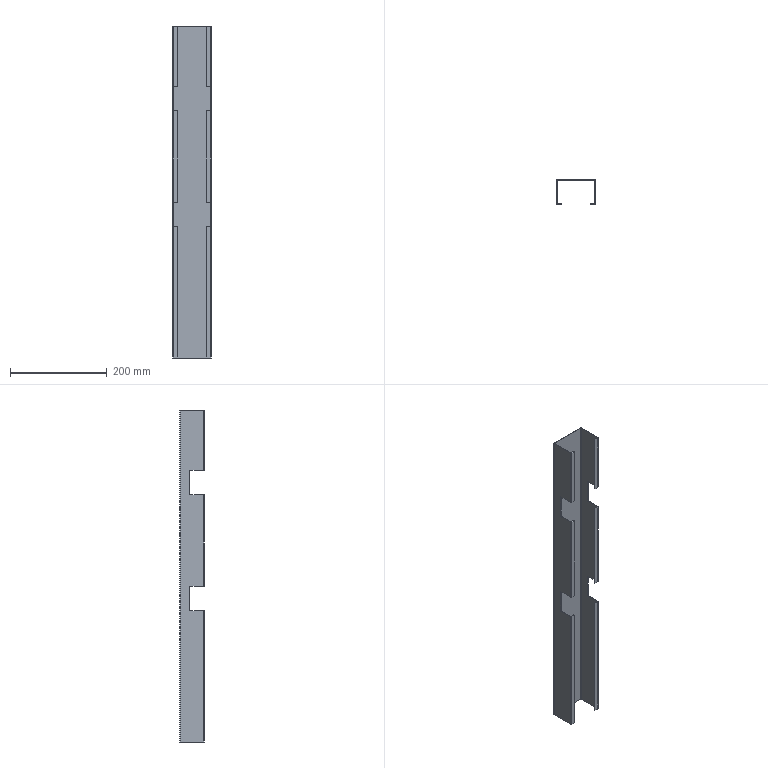Part | SolidWorks | features ICE 2, FlatPattern 1, SMBaseFlange 1, SheetMetal 1, WeldmentFeature 1 | 1 solid | 86 faces | box 80 x 51 x 687 mm | volume 188870 mm3 | plane 70 | cylinder 16 | commonest cylinder face diameters 0.4 x8 3.4 x8